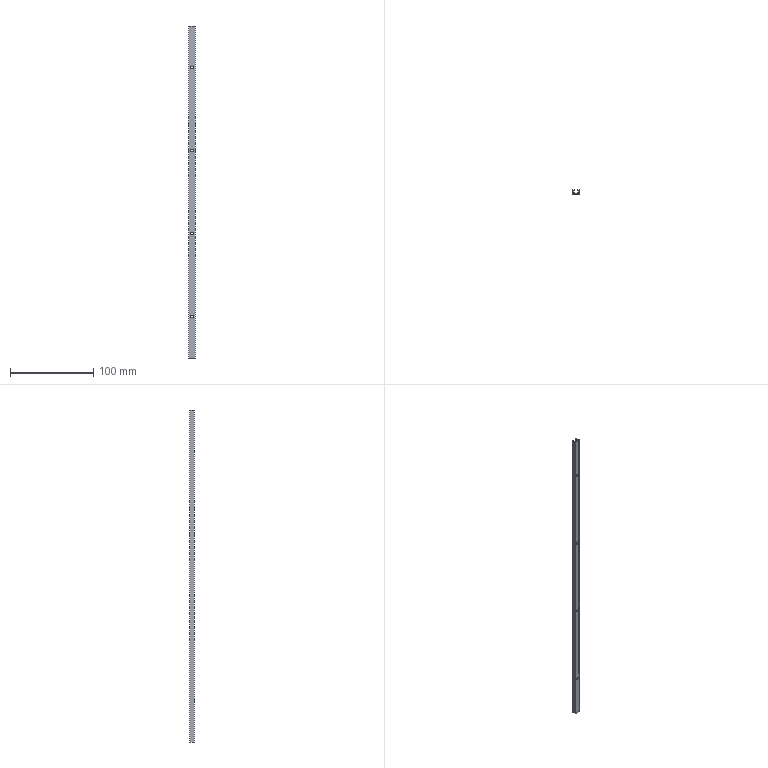Part | SolidWorks | features BaseBody 1 | 1 solid | 26 faces | box 8 x 5 x 400 mm | volume 7551 mm3 | plane 18 | cylinder 8 | commonest cylinder face diameters 3 x8
STEP:
#1=CARTESIAN_POINT('',(0.,0.9,326.5));
#2=VERTEX_POINT('',#1);
#3=CARTESIAN_POINT('',(0.,0.9,323.5));
#4=VERTEX_POINT('',#3);
#5=CARTESIAN_POINT('',(0.,0.9,325.));
#6=DIRECTION('',(0.,-1.,0.));
#7=DIRECTION('',(0.,0.,-1.));
#8=AXIS2_PLACEMENT_3D('',#5,#6,#7);
#9=CIRCLE('',#8,1.5);
#10=EDGE_CURVE('',#2,#4,#9,.T.);
#11=ORIENTED_EDGE('',*,*,#10,.F.);
#12=CARTESIAN_POINT('',(0.,0.,326.5));
#13=VERTEX_POINT('',#12);
#14=CARTESIAN_POINT('',(0.,4.,326.5));
#15=DIRECTION('',(0.,-1.,0.));
#16=VECTOR('',#15,1000.);
#17=LINE('',#14,#16);
#18=EDGE_CURVE('',#2,#13,#17,.T.);
#19=ORIENTED_EDGE('',*,*,#18,.T.);
#20=CARTESIAN_POINT('',(0.,0.,323.5));
#21=VERTEX_POINT('',#20);
#22=CARTESIAN_POINT('',(0.,0.,325.));
#23=DIRECTION('',(0.,1.,0.));
#24=DIRECTION('',(0.,0.,-1.));
#25=AXIS2_PLACEMENT_3D('',#22,#23,#24);
#26=CIRCLE('',#25,1.5);
#27=EDGE_CURVE('',#21,#13,#26,.T.);
#28=ORIENTED_EDGE('',*,*,#27,.F.);
#29=CARTESIAN_POINT('',(0.,4.,323.5));
#30=DIRECTION('',(0.,-1.,0.));
#31=VECTOR('',#30,1000.);
#32=LINE('',#29,#31);
#33=EDGE_CURVE('',#4,#21,#32,.T.);
#34=ORIENTED_EDGE('',*,*,#33,.F.);
#35=EDGE_LOOP('',(#11,#19,#28,#34));
#36=FACE_OUTER_BOUND('',#35,.T.);
#37=CARTESIAN_POINT('',(0.,4.,325.));
#38=DIRECTION('',(0.,-1.,0.));
#39=DIRECTION('',(0.,0.,-1.));
#40=AXIS2_PLACEMENT_3D('',#37,#38,#39);
#41=CYLINDRICAL_SURFACE('',#40,1.5);
#42=ADVANCED_FACE('',(#36),#41,.F.);
#43=CARTESIAN_POINT('',(0.,0.9,226.5));
#44=VERTEX_POINT('',#43);
#45=CARTESIAN_POINT('',(0.,0.9,223.5));
#46=VERTEX_POINT('',#45);
#47=CARTESIAN_POINT('',(0.,0.9,225.));
#48=DIRECTION('',(0.,-1.,0.));
#49=DIRECTION('',(0.,0.,-1.));
#50=AXIS2_PLACEMENT_3D('',#47,#48,#49);
#51=CIRCLE('',#50,1.5);
#52=EDGE_CURVE('',#44,#46,#51,.T.);
#53=ORIENTED_EDGE('',*,*,#52,.F.);
#54=CARTESIAN_POINT('',(0.,0.,226.5));
#55=VERTEX_POINT('',#54);
#56=CARTESIAN_POINT('',(0.,4.,226.5));
#57=DIRECTION('',(0.,-1.,0.));
#58=VECTOR('',#57,1000.);
#59=LINE('',#56,#58);
#60=EDGE_CURVE('',#44,#55,#59,.T.);
#61=ORIENTED_EDGE('',*,*,#60,.T.);
#62=CARTESIAN_POINT('',(0.,0.,223.5));
#63=VERTEX_POINT('',#62);
#64=CARTESIAN_POINT('',(0.,0.,225.));
#65=DIRECTION('',(0.,1.,0.));
#66=DIRECTION('',(0.,0.,-1.));
#67=AXIS2_PLACEMENT_3D('',#64,#65,#66);
#68=CIRCLE('',#67,1.5);
#69=EDGE_CURVE('',#63,#55,#68,.T.);
#70=ORIENTED_EDGE('',*,*,#69,.F.);
#71=CARTESIAN_POINT('',(0.,4.,223.5));
#72=DIRECTION('',(0.,-1.,0.));
#73=VECTOR('',#72,1000.);
#74=LINE('',#71,#73);
#75=EDGE_CURVE('',#46,#63,#74,.T.);
#76=ORIENTED_EDGE('',*,*,#75,.F.);
#77=EDGE_LOOP('',(#53,#61,#70,#76));
#78=FACE_OUTER_BOUND('',#77,.T.);
#79=CARTESIAN_POINT('',(0.,4.,225.));
#80=DIRECTION('',(0.,-1.,0.));
#81=DIRECTION('',(0.,0.,-1.));
#82=AXIS2_PLACEMENT_3D('',#79,#80,#81);
#83=CYLINDRICAL_SURFACE('',#82,1.5);
#84=ADVANCED_FACE('',(#78),#83,.F.);
#85=CARTESIAN_POINT('',(0.,0.9,126.5));
#86=VERTEX_POINT('',#85);
#87=CARTESIAN_POINT('',(0.,0.9,123.5));
#88=VERTEX_POINT('',#87);
#89=CARTESIAN_POINT('',(0.,0.9,125.));
#90=DIRECTION('',(0.,-1.,0.));
#91=DIRECTION('',(0.,0.,-1.));
#92=AXIS2_PLACEMENT_3D('',#89,#90,#91);
#93=CIRCLE('',#92,1.5);
#94=EDGE_CURVE('',#86,#88,#93,.T.);
#95=ORIENTED_EDGE('',*,*,#94,.F.);
#96=CARTESIAN_POINT('',(0.,0.,126.5));
#97=VERTEX_POINT('',#96);
#98=CARTESIAN_POINT('',(0.,4.,126.5));
#99=DIRECTION('',(0.,-1.,0.));
#100=VECTOR('',#99,1000.);
#101=LINE('',#98,#100);
#102=EDGE_CURVE('',#86,#97,#101,.T.);
#103=ORIENTED_EDGE('',*,*,#102,.T.);
#104=CARTESIAN_POINT('',(0.,0.,123.5));
#105=VERTEX_POINT('',#104);
#106=CARTESIAN_POINT('',(0.,0.,125.));
#107=DIRECTION('',(0.,1.,0.));
#108=DIRECTION('',(0.,0.,-1.));
#109=AXIS2_PLACEMENT_3D('',#106,#107,#108);
#110=CIRCLE('',#109,1.5);
#111=EDGE_CURVE('',#105,#97,#110,.T.);
#112=ORIENTED_EDGE('',*,*,#111,.F.);
#113=CARTESIAN_POINT('',(0.,4.,123.5));
#114=DIRECTION('',(0.,-1.,0.));
#115=VECTOR('',#114,1000.);
#116=LINE('',#113,#115);
#117=EDGE_CURVE('',#88,#105,#116,.T.);
#118=ORIENTED_EDGE('',*,*,#117,.F.);
#119=EDGE_LOOP('',(#95,#103,#112,#118));
#120=FACE_OUTER_BOUND('',#119,.T.);
#121=CARTESIAN_POINT('',(0.,4.,125.));
#122=DIRECTION('',(0.,-1.,0.));
#123=DIRECTION('',(0.,0.,-1.));
#124=AXIS2_PLACEMENT_3D('',#121,#122,#123);
#125=CYLINDRICAL_SURFACE('',#124,1.5);
#126=ADVANCED_FACE('',(#120),#125,.F.);
#127=CARTESIAN_POINT('',(0.,0.9,26.5));
#128=VERTEX_POINT('',#127);
#129=CARTESIAN_POINT('',(0.,0.9,23.5));
#130=VERTEX_POINT('',#129);
#131=CARTESIAN_POINT('',(0.,0.9,25.));
#132=DIRECTION('',(0.,-1.,0.));
#133=DIRECTION('',(0.,0.,-1.));
#134=AXIS2_PLACEMENT_3D('',#131,#132,#133);
#135=CIRCLE('',#134,1.5);
#136=EDGE_CURVE('',#128,#130,#135,.T.);
#137=ORIENTED_EDGE('',*,*,#136,.F.);
#138=CARTESIAN_POINT('',(0.,0.,26.5));
#139=VERTEX_POINT('',#138);
#140=CARTESIAN_POINT('',(0.,4.,26.5));
#141=DIRECTION('',(0.,-1.,0.));
#142=VECTOR('',#141,1000.);
#143=LINE('',#140,#142);
#144=EDGE_CURVE('',#128,#139,#143,.T.);
#145=ORIENTED_EDGE('',*,*,#144,.T.);
#146=CARTESIAN_POINT('',(0.,0.,23.5));
#147=VERTEX_POINT('',#146);
#148=CARTESIAN_POINT('',(0.,0.,25.));
#149=DIRECTION('',(0.,1.,0.));
#150=DIRECTION('',(0.,0.,-1.));
#151=AXIS2_PLACEMENT_3D('',#148,#149,#150);
#152=CIRCLE('',#151,1.5);
#153=EDGE_CURVE('',#147,#139,#152,.T.);
#154=ORIENTED_EDGE('',*,*,#153,.F.);
#155=CARTESIAN_POINT('',(0.,4.,23.5));
#156=DIRECTION('',(0.,-1.,0.));
#157=VECTOR('',#156,1000.);
#158=LINE('',#155,#157);
#159=EDGE_CURVE('',#130,#147,#158,.T.);
#160=ORIENTED_EDGE('',*,*,#159,.F.);
#161=EDGE_LOOP('',(#137,#145,#154,#160));
#162=FACE_OUTER_BOUND('',#161,.T.);
#163=CARTESIAN_POINT('',(0.,4.,25.));
#164=DIRECTION('',(0.,-1.,0.));
#165=DIRECTION('',(0.,0.,-1.));
#166=AXIS2_PLACEMENT_3D('',#163,#164,#165);
#167=CYLINDRICAL_SURFACE('',#166,1.5);
#168=ADVANCED_FACE('',(#162),#167,.F.);
#169=ORIENTED_EDGE('',*,*,#27,.T.);
#170=CARTESIAN_POINT('',(0.,0.,325.));
#171=DIRECTION('',(0.,1.,0.));
#172=DIRECTION('',(0.,0.,-1.));
#173=AXIS2_PLACEMENT_3D('',#170,#171,#172);
#174=CIRCLE('',#173,1.5);
#175=EDGE_CURVE('',#13,#21,#174,.T.);
#176=ORIENTED_EDGE('',*,*,#175,.T.);
#177=EDGE_LOOP('',(#169,#176));
#178=FACE_BOUND('',#177,.T.);
#179=ORIENTED_EDGE('',*,*,#69,.T.);
#180=CARTESIAN_POINT('',(0.,0.,225.));
#181=DIRECTION('',(0.,1.,0.));
#182=DIRECTION('',(0.,0.,-1.));
#183=AXIS2_PLACEMENT_3D('',#180,#181,#182);
#184=CIRCLE('',#183,1.5);
#185=EDGE_CURVE('',#55,#63,#184,.T.);
#186=ORIENTED_EDGE('',*,*,#185,.T.);
#187=EDGE_LOOP('',(#179,#186));
#188=FACE_BOUND('',#187,.T.);
#189=ORIENTED_EDGE('',*,*,#111,.T.);
#190=CARTESIAN_POINT('',(0.,0.,125.));
#191=DIRECTION('',(0.,1.,0.));
#192=DIRECTION('',(0.,0.,-1.));
#193=AXIS2_PLACEMENT_3D('',#190,#191,#192);
#194=CIRCLE('',#193,1.5);
#195=EDGE_CURVE('',#97,#105,#194,.T.);
#196=ORIENTED_EDGE('',*,*,#195,.T.);
#197=EDGE_LOOP('',(#189,#196));
#198=FACE_BOUND('',#197,.T.);
#199=ORIENTED_EDGE('',*,*,#153,.T.);
#200=CARTESIAN_POINT('',(0.,0.,25.));
#201=DIRECTION('',(0.,1.,0.));
#202=DIRECTION('',(0.,0.,-1.));
#203=AXIS2_PLACEMENT_3D('',#200,#201,#202);
#204=CIRCLE('',#203,1.5);
#205=EDGE_CURVE('',#139,#147,#204,.T.);
#206=ORIENTED_EDGE('',*,*,#205,.T.);
#207=EDGE_LOOP('',(#199,#206));
#208=FACE_BOUND('',#207,.T.);
#209=CARTESIAN_POINT('',(-4.,0.,-25.));
#210=VERTEX_POINT('',#209);
#211=CARTESIAN_POINT('',(4.,0.,-25.));
#212=VERTEX_POINT('',#211);
#213=CARTESIAN_POINT('',(-4.,0.,-25.));
#214=DIRECTION('',(1.,0.,0.));
#215=VECTOR('',#214,1000.);
#216=LINE('',#213,#215);
#217=EDGE_CURVE('',#210,#212,#216,.T.);
#218=ORIENTED_EDGE('',*,*,#217,.T.);
#219=CARTESIAN_POINT('',(4.,0.,375.));
#220=VERTEX_POINT('',#219);
#221=CARTESIAN_POINT('',(4.,0.,0.));
#222=DIRECTION('',(0.,0.,1.));
#223=VECTOR('',#222,1000.);
#224=LINE('',#221,#223);
#225=EDGE_CURVE('',#212,#220,#224,.T.);
#226=ORIENTED_EDGE('',*,*,#225,.T.);
#227=CARTESIAN_POINT('',(-4.,0.,375.));
#228=VERTEX_POINT('',#227);
#229=CARTESIAN_POINT('',(-4.,0.,375.));
#230=DIRECTION('',(-1.,0.,0.));
#231=VECTOR('',#230,1000.);
#232=LINE('',#229,#231);
#233=EDGE_CURVE('',#220,#228,#232,.T.);
#234=ORIENTED_EDGE('',*,*,#233,.T.);
#235=CARTESIAN_POINT('',(-4.,0.,0.));
#236=DIRECTION('',(0.,0.,-1.));
#237=VECTOR('',#236,1000.);
#238=LINE('',#235,#237);
#239=EDGE_CURVE('',#228,#210,#238,.T.);
#240=ORIENTED_EDGE('',*,*,#239,.T.);
#241=EDGE_LOOP('',(#218,#226,#234,#240));
#242=FACE_OUTER_BOUND('',#241,.T.);
#243=CARTESIAN_POINT('',(-4.,0.,0.));
#244=DIRECTION('',(0.,-1.,0.));
#245=DIRECTION('',(0.,0.,-1.));
#246=AXIS2_PLACEMENT_3D('',#243,#244,#245);
#247=PLANE('',#246);
#248=ADVANCED_FACE('',(#178,#188,#198,#208,#242),#247,.T.);
#249=ORIENTED_EDGE('',*,*,#18,.F.);
#250=CARTESIAN_POINT('',(0.,0.9,325.));
#251=DIRECTION('',(0.,-1.,0.));
#252=DIRECTION('',(0.,0.,-1.));
#253=AXIS2_PLACEMENT_3D('',#250,#251,#252);
#254=CIRCLE('',#253,1.5);
#255=EDGE_CURVE('',#4,#2,#254,.T.);
#256=ORIENTED_EDGE('',*,*,#255,.F.);
#257=ORIENTED_EDGE('',*,*,#33,.T.);
#258=ORIENTED_EDGE('',*,*,#175,.F.);
#259=EDGE_LOOP('',(#249,#256,#257,#258));
#260=FACE_OUTER_BOUND('',#259,.T.);
#261=CARTESIAN_POINT('',(0.,4.,325.));
#262=DIRECTION('',(0.,-1.,0.));
#263=DIRECTION('',(0.,0.,-1.));
#264=AXIS2_PLACEMENT_3D('',#261,#262,#263);
#265=CYLINDRICAL_SURFACE('',#264,1.5);
#266=ADVANCED_FACE('',(#260),#265,.F.);
#267=ORIENTED_EDGE('',*,*,#60,.F.);
#268=CARTESIAN_POINT('',(0.,0.9,225.));
#269=DIRECTION('',(0.,-1.,0.));
#270=DIRECTION('',(0.,0.,-1.));
#271=AXIS2_PLACEMENT_3D('',#268,#269,#270);
#272=CIRCLE('',#271,1.5);
#273=EDGE_CURVE('',#46,#44,#272,.T.);
#274=ORIENTED_EDGE('',*,*,#273,.F.);
#275=ORIENTED_EDGE('',*,*,#75,.T.);
#276=ORIENTED_EDGE('',*,*,#185,.F.);
#277=EDGE_LOOP('',(#267,#274,#275,#276));
#278=FACE_OUTER_BOUND('',#277,.T.);
#279=CARTESIAN_POINT('',(0.,4.,225.));
#280=DIRECTION('',(0.,-1.,0.));
#281=DIRECTION('',(0.,0.,-1.));
#282=AXIS2_PLACEMENT_3D('',#279,#280,#281);
#283=CYLINDRICAL_SURFACE('',#282,1.5);
#284=ADVANCED_FACE('',(#278),#283,.F.);
#285=ORIENTED_EDGE('',*,*,#102,.F.);
#286=CARTESIAN_POINT('',(0.,0.9,125.));
#287=DIRECTION('',(0.,-1.,0.));
#288=DIRECTION('',(0.,0.,-1.));
#289=AXIS2_PLACEMENT_3D('',#286,#287,#288);
#290=CIRCLE('',#289,1.5);
#291=EDGE_CURVE('',#88,#86,#290,.T.);
#292=ORIENTED_EDGE('',*,*,#291,.F.);
#293=ORIENTED_EDGE('',*,*,#117,.T.);
#294=ORIENTED_EDGE('',*,*,#195,.F.);
#295=EDGE_LOOP('',(#285,#292,#293,#294));
#296=FACE_OUTER_BOUND('',#295,.T.);
#297=CARTESIAN_POINT('',(0.,4.,125.));
#298=DIRECTION('',(0.,-1.,0.));
#299=DIRECTION('',(0.,0.,-1.));
#300=AXIS2_PLACEMENT_3D('',#297,#298,#299);
#301=CYLINDRICAL_SURFACE('',#300,1.5);
#302=ADVANCED_FACE('',(#296),#301,.F.);
#303=ORIENTED_EDGE('',*,*,#144,.F.);
#304=CARTESIAN_POINT('',(0.,0.9,25.));
#305=DIRECTION('',(0.,-1.,0.));
#306=DIRECTION('',(0.,0.,-1.));
#307=AXIS2_PLACEMENT_3D('',#304,#305,#306);
#308=CIRCLE('',#307,1.5);
#309=EDGE_CURVE('',#130,#128,#308,.T.);
#310=ORIENTED_EDGE('',*,*,#309,.F.);
#311=ORIENTED_EDGE('',*,*,#159,.T.);
#312=ORIENTED_EDGE('',*,*,#205,.F.);
#313=EDGE_LOOP('',(#303,#310,#311,#312));
#314=FACE_OUTER_BOUND('',#313,.T.);
#315=CARTESIAN_POINT('',(0.,4.,25.));
#316=DIRECTION('',(0.,-1.,0.));
#317=DIRECTION('',(0.,0.,-1.));
#318=AXIS2_PLACEMENT_3D('',#315,#316,#317);
#319=CYLINDRICAL_SURFACE('',#318,1.5);
#320=ADVANCED_FACE('',(#314),#319,.F.);
#321=CARTESIAN_POINT('',(4.,5.,375.));
#322=VERTEX_POINT('',#321);
#323=CARTESIAN_POINT('',(4.,0.,375.));
#324=DIRECTION('',(0.,-1.,0.));
#325=VECTOR('',#324,1000.);
#326=LINE('',#323,#325);
#327=EDGE_CURVE('',#322,#220,#326,.T.);
#328=ORIENTED_EDGE('',*,*,#327,.T.);
#329=ORIENTED_EDGE('',*,*,#225,.F.);
#330=CARTESIAN_POINT('',(4.,5.,-25.));
#331=VERTEX_POINT('',#330);
#332=CARTESIAN_POINT('',(4.,0.,-25.));
#333=DIRECTION('',(0.,1.,0.));
#334=VECTOR('',#333,1000.);
#335=LINE('',#332,#334);
#336=EDGE_CURVE('',#212,#331,#335,.T.);
#337=ORIENTED_EDGE('',*,*,#336,.T.);
#338=CARTESIAN_POINT('',(4.,5.,0.));
#339=DIRECTION('',(0.,0.,1.));
#340=VECTOR('',#339,1000.);
#341=LINE('',#338,#340);
#342=EDGE_CURVE('',#331,#322,#341,.T.);
#343=ORIENTED_EDGE('',*,*,#342,.T.);
#344=EDGE_LOOP('',(#328,#329,#337,#343));
#345=FACE_OUTER_BOUND('',#344,.T.);
#346=CARTESIAN_POINT('',(4.,0.,0.));
#347=DIRECTION('',(1.,0.,0.));
#348=DIRECTION('',(0.,0.,-1.));
#349=AXIS2_PLACEMENT_3D('',#346,#347,#348);
#350=PLANE('',#349);
#351=ADVANCED_FACE('',(#345),#350,.T.);
#352=ORIENTED_EDGE('',*,*,#217,.F.);
#353=CARTESIAN_POINT('',(-4.,5.,-25.));
#354=VERTEX_POINT('',#353);
#355=CARTESIAN_POINT('',(-4.,0.,-25.));
#356=DIRECTION('',(0.,-1.,0.));
#357=VECTOR('',#356,1000.);
#358=LINE('',#355,#357);
#359=EDGE_CURVE('',#354,#210,#358,.T.);
#360=ORIENTED_EDGE('',*,*,#359,.F.);
#361=CARTESIAN_POINT('',(-2.1,5.,-25.));
#362=VERTEX_POINT('',#361);
#363=CARTESIAN_POINT('',(0.,5.,-25.));
#364=DIRECTION('',(-1.,0.,0.));
#365=VECTOR('',#364,1000.);
#366=LINE('',#363,#365);
#367=EDGE_CURVE('',#362,#354,#366,.T.);
#368=ORIENTED_EDGE('',*,*,#367,.F.);
#369=CARTESIAN_POINT('',(-2.1,4.2,-25.));
#370=VERTEX_POINT('',#369);
#371=CARTESIAN_POINT('',(-2.1,4.2,-25.));
#372=DIRECTION('',(0.,1.,0.));
#373=VECTOR('',#372,1000.);
#374=LINE('',#371,#373);
#375=EDGE_CURVE('',#370,#362,#374,.T.);
#376=ORIENTED_EDGE('',*,*,#375,.F.);
#377=CARTESIAN_POINT('',(-2.9,4.2,-25.));
#378=VERTEX_POINT('',#377);
#379=CARTESIAN_POINT('',(-2.9,4.2,-25.));
#380=DIRECTION('',(1.,0.,0.));
#381=VECTOR('',#380,1000.);
#382=LINE('',#379,#381);
#383=EDGE_CURVE('',#378,#370,#382,.T.);
#384=ORIENTED_EDGE('',*,*,#383,.F.);
#385=CARTESIAN_POINT('',(-2.9,1.8,-25.));
#386=VERTEX_POINT('',#385);
#387=CARTESIAN_POINT('',(-2.9,0.,-25.));
#388=DIRECTION('',(0.,1.,0.));
#389=VECTOR('',#388,1000.);
#390=LINE('',#387,#389);
#391=EDGE_CURVE('',#386,#378,#390,.T.);
#392=ORIENTED_EDGE('',*,*,#391,.F.);
#393=CARTESIAN_POINT('',(-2.1,1.8,-25.));
#394=VERTEX_POINT('',#393);
#395=CARTESIAN_POINT('',(-2.1,1.8,-25.));
#396=DIRECTION('',(-1.,0.,0.));
#397=VECTOR('',#396,1000.);
#398=LINE('',#395,#397);
#399=EDGE_CURVE('',#394,#386,#398,.T.);
#400=ORIENTED_EDGE('',*,*,#399,.F.);
#401=CARTESIAN_POINT('',(-2.1,0.9,-25.));
#402=VERTEX_POINT('',#401);
#403=CARTESIAN_POINT('',(-2.1,0.9,-25.));
#404=DIRECTION('',(0.,1.,0.));
#405=VECTOR('',#404,1000.);
#406=LINE('',#403,#405);
#407=EDGE_CURVE('',#402,#394,#406,.T.);
#408=ORIENTED_EDGE('',*,*,#407,.F.);
#409=CARTESIAN_POINT('',(2.1,0.9,-25.));
#410=VERTEX_POINT('',#409);
#411=CARTESIAN_POINT('',(0.,0.9,-25.));
#412=DIRECTION('',(-1.,0.,0.));
#413=VECTOR('',#412,1000.);
#414=LINE('',#411,#413);
#415=EDGE_CURVE('',#410,#402,#414,.T.);
#416=ORIENTED_EDGE('',*,*,#415,.F.);
#417=CARTESIAN_POINT('',(2.1,1.8,-25.));
#418=VERTEX_POINT('',#417);
#419=CARTESIAN_POINT('',(2.1,1.8,-25.));
#420=DIRECTION('',(0.,-1.,0.));
#421=VECTOR('',#420,1000.);
#422=LINE('',#419,#421);
#423=EDGE_CURVE('',#418,#410,#422,.T.);
#424=ORIENTED_EDGE('',*,*,#423,.F.);
#425=CARTESIAN_POINT('',(2.9,1.8,-25.));
#426=VERTEX_POINT('',#425);
#427=CARTESIAN_POINT('',(2.9,1.8,-25.));
#428=DIRECTION('',(-1.,0.,0.));
#429=VECTOR('',#428,1000.);
#430=LINE('',#427,#429);
#431=EDGE_CURVE('',#426,#418,#430,.T.);
#432=ORIENTED_EDGE('',*,*,#431,.F.);
#433=CARTESIAN_POINT('',(2.9,4.2,-25.));
#434=VERTEX_POINT('',#433);
#435=CARTESIAN_POINT('',(2.9,0.,-25.));
#436=DIRECTION('',(0.,-1.,0.));
#437=VECTOR('',#436,1000.);
#438=LINE('',#435,#437);
#439=EDGE_CURVE('',#434,#426,#438,.T.);
#440=ORIENTED_EDGE('',*,*,#439,.F.);
#441=CARTESIAN_POINT('',(2.1,4.2,-25.));
#442=VERTEX_POINT('',#441);
#443=CARTESIAN_POINT('',(2.1,4.2,-25.));
#444=DIRECTION('',(1.,0.,0.));
#445=VECTOR('',#444,1000.);
#446=LINE('',#443,#445);
#447=EDGE_CURVE('',#442,#434,#446,.T.);
#448=ORIENTED_EDGE('',*,*,#447,.F.);
#449=CARTESIAN_POINT('',(2.1,5.,-25.));
#450=VERTEX_POINT('',#449);
#451=CARTESIAN_POINT('',(2.1,5.,-25.));
#452=DIRECTION('',(0.,-1.,0.));
#453=VECTOR('',#452,1000.);
#454=LINE('',#451,#453);
#455=EDGE_CURVE('',#450,#442,#454,.T.);
#456=ORIENTED_EDGE('',*,*,#455,.F.);
#457=CARTESIAN_POINT('',(0.,5.,-25.));
#458=DIRECTION('',(-1.,0.,0.));
#459=VECTOR('',#458,1000.);
#460=LINE('',#457,#459);
#461=EDGE_CURVE('',#331,#450,#460,.T.);
#462=ORIENTED_EDGE('',*,*,#461,.F.);
#463=ORIENTED_EDGE('',*,*,#336,.F.);
#464=EDGE_LOOP('',(#352,#360,#368,#376,#384,#392,#400,#408,#416,#424,#432,#440,#448,#456,#462,#463));
#465=FACE_OUTER_BOUND('',#464,.T.);
#466=CARTESIAN_POINT('',(0.,0.,-25.));
#467=DIRECTION('',(0.,0.,1.));
#468=DIRECTION('',(1.,0.,0.));
#469=AXIS2_PLACEMENT_3D('',#466,#467,#468);
#470=PLANE('',#469);
#471=ADVANCED_FACE('',(#465),#470,.F.);
#472=CARTESIAN_POINT('',(-4.,5.,375.));
#473=VERTEX_POINT('',#472);
#474=CARTESIAN_POINT('',(-4.,5.,375.));
#475=DIRECTION('',(0.,1.,0.));
#476=VECTOR('',#475,1000.);
#477=LINE('',#474,#476);
#478=EDGE_CURVE('',#228,#473,#477,.T.);
#479=ORIENTED_EDGE('',*,*,#478,.T.);
#480=CARTESIAN_POINT('',(-4.,5.,0.));
#481=DIRECTION('',(0.,0.,-1.));
#482=VECTOR('',#481,1000.);
#483=LINE('',#480,#482);
#484=EDGE_CURVE('',#473,#354,#483,.T.);
#485=ORIENTED_EDGE('',*,*,#484,.T.);
#486=ORIENTED_EDGE('',*,*,#359,.T.);
#487=ORIENTED_EDGE('',*,*,#239,.F.);
#488=EDGE_LOOP('',(#479,#485,#486,#487));
#489=FACE_OUTER_BOUND('',#488,.T.);
#490=CARTESIAN_POINT('',(-4.,5.,0.));
#491=DIRECTION('',(-1.,0.,0.));
#492=DIRECTION('',(0.,0.,1.));
#493=AXIS2_PLACEMENT_3D('',#490,#491,#492);
#494=PLANE('',#493);
#495=ADVANCED_FACE('',(#489),#494,.T.);
#496=CARTESIAN_POINT('',(2.1,1.8,375.));
#497=VERTEX_POINT('',#496);
#498=CARTESIAN_POINT('',(2.9,1.8,375.));
#499=VERTEX_POINT('',#498);
#500=CARTESIAN_POINT('',(2.9,1.8,375.));
#501=DIRECTION('',(1.,0.,0.));
#502=VECTOR('',#501,1000.);
#503=LINE('',#500,#502);
#504=EDGE_CURVE('',#497,#499,#503,.T.);
#505=ORIENTED_EDGE('',*,*,#504,.F.);
#506=CARTESIAN_POINT('',(2.1,0.9,375.));
#507=VERTEX_POINT('',#506);
#508=CARTESIAN_POINT('',(2.1,1.8,375.));
#509=DIRECTION('',(0.,1.,0.));
#510=VECTOR('',#509,1000.);
#511=LINE('',#508,#510);
#512=EDGE_CURVE('',#507,#497,#511,.T.);
#513=ORIENTED_EDGE('',*,*,#512,.F.);
#514=CARTESIAN_POINT('',(-2.1,0.9,375.));
#515=VERTEX_POINT('',#514);
#516=CARTESIAN_POINT('',(0.,0.9,375.));
#517=DIRECTION('',(-1.,0.,0.));
#518=VECTOR('',#517,1000.);
#519=LINE('',#516,#518);
#520=EDGE_CURVE('',#507,#515,#519,.T.);
#521=ORIENTED_EDGE('',*,*,#520,.T.);
#522=CARTESIAN_POINT('',(-2.1,1.8,375.));
#523=VERTEX_POINT('',#522);
#524=CARTESIAN_POINT('',(-2.1,0.9,375.));
#525=DIRECTION('',(0.,-1.,0.));
#526=VECTOR('',#525,1000.);
#527=LINE('',#524,#526);
#528=EDGE_CURVE('',#523,#515,#527,.T.);
#529=ORIENTED_EDGE('',*,*,#528,.F.);
#530=CARTESIAN_POINT('',(-2.9,1.8,375.));
#531=VERTEX_POINT('',#530);
#532=CARTESIAN_POINT('',(-2.1,1.8,375.));
#533=DIRECTION('',(1.,0.,0.));
#534=VECTOR('',#533,1000.);
#535=LINE('',#532,#534);
#536=EDGE_CURVE('',#531,#523,#535,.T.);
#537=ORIENTED_EDGE('',*,*,#536,.F.);
#538=CARTESIAN_POINT('',(-2.9,4.2,375.));
#539=VERTEX_POINT('',#538);
#540=CARTESIAN_POINT('',(-2.9,0.,375.));
#541=DIRECTION('',(0.,1.,0.));
#542=VECTOR('',#541,1000.);
#543=LINE('',#540,#542);
#544=EDGE_CURVE('',#531,#539,#543,.T.);
#545=ORIENTED_EDGE('',*,*,#544,.T.);
#546=CARTESIAN_POINT('',(-2.1,4.2,375.));
#547=VERTEX_POINT('',#546);
#548=CARTESIAN_POINT('',(-2.9,4.2,375.));
#549=DIRECTION('',(-1.,0.,0.));
#550=VECTOR('',#549,1000.);
#551=LINE('',#548,#550);
#552=EDGE_CURVE('',#547,#539,#551,.T.);
#553=ORIENTED_EDGE('',*,*,#552,.F.);
#554=CARTESIAN_POINT('',(-2.1,5.,375.));
#555=VERTEX_POINT('',#554);
#556=CARTESIAN_POINT('',(-2.1,4.2,375.));
#557=DIRECTION('',(0.,-1.,0.));
#558=VECTOR('',#557,1000.);
#559=LINE('',#556,#558);
#560=EDGE_CURVE('',#555,#547,#559,.T.);
#561=ORIENTED_EDGE('',*,*,#560,.F.);
#562=CARTESIAN_POINT('',(0.,5.,375.));
#563=DIRECTION('',(-1.,0.,0.));
#564=VECTOR('',#563,1000.);
#565=LINE('',#562,#564);
#566=EDGE_CURVE('',#555,#473,#565,.T.);
#567=ORIENTED_EDGE('',*,*,#566,.T.);
#568=ORIENTED_EDGE('',*,*,#478,.F.);
#569=ORIENTED_EDGE('',*,*,#233,.F.);
#570=ORIENTED_EDGE('',*,*,#327,.F.);
#571=CARTESIAN_POINT('',(2.1,5.,375.));
#572=VERTEX_POINT('',#571);
#573=CARTESIAN_POINT('',(0.,5.,375.));
#574=DIRECTION('',(-1.,0.,0.));
#575=VECTOR('',#574,1000.);
#576=LINE('',#573,#575);
#577=EDGE_CURVE('',#322,#572,#576,.T.);
#578=ORIENTED_EDGE('',*,*,#577,.T.);
#579=CARTESIAN_POINT('',(2.1,4.2,375.));
#580=VERTEX_POINT('',#579);
#581=CARTESIAN_POINT('',(2.1,5.,375.));
#582=DIRECTION('',(0.,1.,0.));
#583=VECTOR('',#582,1000.);
#584=LINE('',#581,#583);
#585=EDGE_CURVE('',#580,#572,#584,.T.);
#586=ORIENTED_EDGE('',*,*,#585,.F.);
#587=CARTESIAN_POINT('',(2.9,4.2,375.));
#588=VERTEX_POINT('',#587);
#589=CARTESIAN_POINT('',(2.1,4.2,375.));
#590=DIRECTION('',(-1.,0.,0.));
#591=VECTOR('',#590,1000.);
#592=LINE('',#589,#591);
#593=EDGE_CURVE('',#588,#580,#592,.T.);
#594=ORIENTED_EDGE('',*,*,#593,.F.);
#595=CARTESIAN_POINT('',(2.9,0.,375.));
#596=DIRECTION('',(0.,-1.,0.));
#597=VECTOR('',#596,1000.);
#598=LINE('',#595,#597);
#599=EDGE_CURVE('',#588,#499,#598,.T.);
#600=ORIENTED_EDGE('',*,*,#599,.T.);
#601=EDGE_LOOP('',(#505,#513,#521,#529,#537,#545,#553,#561,#567,#568,#569,#570,#578,#586,#594,#600));
#602=FACE_OUTER_BOUND('',#601,.T.);
#603=CARTESIAN_POINT('',(0.,0.,375.));
#604=DIRECTION('',(0.,0.,1.));
#605=DIRECTION('',(1.,0.,0.));
#606=AXIS2_PLACEMENT_3D('',#603,#604,#605);
#607=PLANE('',#606);
#608=ADVANCED_FACE('',(#602),#607,.T.);
#609=ORIENTED_EDGE('',*,*,#255,.T.);
#610=ORIENTED_EDGE('',*,*,#10,.T.);
#611=EDGE_LOOP('',(#609,#610));
#612=FACE_BOUND('',#611,.T.);
#613=ORIENTED_EDGE('',*,*,#273,.T.);
#614=ORIENTED_EDGE('',*,*,#52,.T.);
#615=EDGE_LOOP('',(#613,#614));
#616=FACE_BOUND('',#615,.T.);
#617=ORIENTED_EDGE('',*,*,#291,.T.);
#618=ORIENTED_EDGE('',*,*,#94,.T.);
#619=EDGE_LOOP('',(#617,#618));
#620=FACE_BOUND('',#619,.T.);
#621=ORIENTED_EDGE('',*,*,#309,.T.);
#622=ORIENTED_EDGE('',*,*,#136,.T.);
#623=EDGE_LOOP('',(#621,#622));
#624=FACE_BOUND('',#623,.T.);
#625=ORIENTED_EDGE('',*,*,#415,.T.);
#626=CARTESIAN_POINT('',(-2.1,0.9,0.));
#627=DIRECTION('',(0.,0.,1.));
#628=VECTOR('',#627,1000.);
#629=LINE('',#626,#628);
#630=EDGE_CURVE('',#402,#515,#629,.T.);
#631=ORIENTED_EDGE('',*,*,#630,.T.);
#632=ORIENTED_EDGE('',*,*,#520,.F.);
#633=CARTESIAN_POINT('',(2.1,0.9,0.));
#634=DIRECTION('',(0.,0.,-1.));
#635=VECTOR('',#634,1000.);
#636=LINE('',#633,#635);
#637=EDGE_CURVE('',#507,#410,#636,.T.);
#638=ORIENTED_EDGE('',*,*,#637,.T.);
#639=EDGE_LOOP('',(#625,#631,#632,#638));
#640=FACE_OUTER_BOUND('',#639,.T.);
#641=CARTESIAN_POINT('',(2.1,0.9,0.));
#642=DIRECTION('',(0.,1.,0.));
#643=DIRECTION('',(0.,0.,1.));
#644=AXIS2_PLACEMENT_3D('',#641,#642,#643);
#645=PLANE('',#644);
#646=ADVANCED_FACE('',(#612,#616,#620,#624,#640),#645,.T.);
#647=ORIENTED_EDGE('',*,*,#577,.F.);
#648=ORIENTED_EDGE('',*,*,#342,.F.);
#649=ORIENTED_EDGE('',*,*,#461,.T.);
#650=CARTESIAN_POINT('',(2.1,5.,0.));
#651=DIRECTION('',(0.,0.,1.));
#652=VECTOR('',#651,1000.);
#653=LINE('',#650,#652);
#654=EDGE_CURVE('',#450,#572,#653,.T.);
#655=ORIENTED_EDGE('',*,*,#654,.T.);
#656=EDGE_LOOP('',(#647,#648,#649,#655));
#657=FACE_OUTER_BOUND('',#656,.T.);
#658=CARTESIAN_POINT('',(4.,5.,0.));
#659=DIRECTION('',(0.,1.,0.));
#660=DIRECTION('',(0.,0.,1.));
#661=AXIS2_PLACEMENT_3D('',#658,#659,#660);
#662=PLANE('',#661);
#663=ADVANCED_FACE('',(#657),#662,.T.);
#664=ORIENTED_EDGE('',*,*,#566,.F.);
#665=CARTESIAN_POINT('',(-2.1,5.,0.));
#666=DIRECTION('',(0.,0.,-1.));
#667=VECTOR('',#666,1000.);
#668=LINE('',#665,#667);
#669=EDGE_CURVE('',#555,#362,#668,.T.);
#670=ORIENTED_EDGE('',*,*,#669,.T.);
#671=ORIENTED_EDGE('',*,*,#367,.T.);
#672=ORIENTED_EDGE('',*,*,#484,.F.);
#673=EDGE_LOOP('',(#664,#670,#671,#672));
#674=FACE_OUTER_BOUND('',#673,.T.);
#675=CARTESIAN_POINT('',(-2.1,5.,0.));
#676=DIRECTION('',(0.,1.,0.));
#677=DIRECTION('',(0.,0.,1.));
#678=AXIS2_PLACEMENT_3D('',#675,#676,#677);
#679=PLANE('',#678);
#680=ADVANCED_FACE('',(#674),#679,.T.);
#681=ORIENTED_EDGE('',*,*,#544,.F.);
#682=CARTESIAN_POINT('',(-2.9,1.8,0.));
#683=DIRECTION('',(0.,0.,-1.));
#684=VECTOR('',#683,1000.);
#685=LINE('',#682,#684);
#686=EDGE_CURVE('',#531,#386,#685,.T.);
#687=ORIENTED_EDGE('',*,*,#686,.T.);
#688=ORIENTED_EDGE('',*,*,#391,.T.);
#689=CARTESIAN_POINT('',(-2.9,4.2,0.));
#690=DIRECTION('',(0.,0.,1.));
#691=VECTOR('',#690,1000.);
#692=LINE('',#689,#691);
#693=EDGE_CURVE('',#378,#539,#692,.T.);
#694=ORIENTED_EDGE('',*,*,#693,.T.);
#695=EDGE_LOOP('',(#681,#687,#688,#694));
#696=FACE_OUTER_BOUND('',#695,.T.);
#697=CARTESIAN_POINT('',(-2.9,1.8,0.));
#698=DIRECTION('',(1.,0.,0.));
#699=DIRECTION('',(0.,0.,-1.));
#700=AXIS2_PLACEMENT_3D('',#697,#698,#699);
#701=PLANE('',#700);
#702=ADVANCED_FACE('',(#696),#701,.T.);
#703=ORIENTED_EDGE('',*,*,#599,.F.);
#704=CARTESIAN_POINT('',(2.9,4.2,0.));
#705=DIRECTION('',(0.,0.,-1.));
#706=VECTOR('',#705,1000.);
#707=LINE('',#704,#706);
#708=EDGE_CURVE('',#588,#434,#707,.T.);
#709=ORIENTED_EDGE('',*,*,#708,.T.);
#710=ORIENTED_EDGE('',*,*,#439,.T.);
#711=CARTESIAN_POINT('',(2.9,1.8,0.));
#712=DIRECTION('',(0.,0.,1.));
#713=VECTOR('',#712,1000.);
#714=LINE('',#711,#713);
#715=EDGE_CURVE('',#426,#499,#714,.T.);
#716=ORIENTED_EDGE('',*,*,#715,.T.);
#717=EDGE_LOOP('',(#703,#709,#710,#716));
#718=FACE_OUTER_BOUND('',#717,.T.);
#719=CARTESIAN_POINT('',(2.9,4.2,0.));
#720=DIRECTION('',(-1.,0.,0.));
#721=DIRECTION('',(0.,0.,1.));
#722=AXIS2_PLACEMENT_3D('',#719,#720,#721);
#723=PLANE('',#722);
#724=ADVANCED_FACE('',(#718),#723,.T.);
#725=ORIENTED_EDGE('',*,*,#528,.T.);
#726=ORIENTED_EDGE('',*,*,#630,.F.);
#727=ORIENTED_EDGE('',*,*,#407,.T.);
#728=CARTESIAN_POINT('',(-2.1,1.8,0.));
#729=DIRECTION('',(0.,0.,1.));
#730=VECTOR('',#729,1000.);
#731=LINE('',#728,#730);
#732=EDGE_CURVE('',#394,#523,#731,.T.);
#733=ORIENTED_EDGE('',*,*,#732,.T.);
#734=EDGE_LOOP('',(#725,#726,#727,#733));
#735=FACE_OUTER_BOUND('',#734,.T.);
#736=CARTESIAN_POINT('',(-2.1,0.9,0.));
#737=DIRECTION('',(1.,0.,0.));
#738=DIRECTION('',(0.,0.,-1.));
#739=AXIS2_PLACEMENT_3D('',#736,#737,#738);
#740=PLANE('',#739);
#741=ADVANCED_FACE('',(#735),#740,.T.);
#742=ORIENTED_EDGE('',*,*,#512,.T.);
#743=CARTESIAN_POINT('',(2.1,1.8,0.));
#744=DIRECTION('',(0.,0.,-1.));
#745=VECTOR('',#744,1000.);
#746=LINE('',#743,#745);
#747=EDGE_CURVE('',#497,#418,#746,.T.);
#748=ORIENTED_EDGE('',*,*,#747,.T.);
#749=ORIENTED_EDGE('',*,*,#423,.T.);
#750=ORIENTED_EDGE('',*,*,#637,.F.);
#751=EDGE_LOOP('',(#742,#748,#749,#750));
#752=FACE_OUTER_BOUND('',#751,.T.);
#753=CARTESIAN_POINT('',(2.1,1.8,0.));
#754=DIRECTION('',(-1.,0.,0.));
#755=DIRECTION('',(0.,0.,1.));
#756=AXIS2_PLACEMENT_3D('',#753,#754,#755);
#757=PLANE('',#756);
#758=ADVANCED_FACE('',(#752),#757,.T.);
#759=ORIENTED_EDGE('',*,*,#585,.T.);
#760=ORIENTED_EDGE('',*,*,#654,.F.);
#761=ORIENTED_EDGE('',*,*,#455,.T.);
#762=CARTESIAN_POINT('',(2.1,4.2,0.));
#763=DIRECTION('',(0.,0.,1.));
#764=VECTOR('',#763,1000.);
#765=LINE('',#762,#764);
#766=EDGE_CURVE('',#442,#580,#765,.T.);
#767=ORIENTED_EDGE('',*,*,#766,.T.);
#768=EDGE_LOOP('',(#759,#760,#761,#767));
#769=FACE_OUTER_BOUND('',#768,.T.);
#770=CARTESIAN_POINT('',(2.1,5.,0.));
#771=DIRECTION('',(-1.,0.,0.));
#772=DIRECTION('',(0.,0.,1.));
#773=AXIS2_PLACEMENT_3D('',#770,#771,#772);
#774=PLANE('',#773);
#775=ADVANCED_FACE('',(#769),#774,.T.);
#776=ORIENTED_EDGE('',*,*,#560,.T.);
#777=CARTESIAN_POINT('',(-2.1,4.2,0.));
#778=DIRECTION('',(0.,0.,-1.));
#779=VECTOR('',#778,1000.);
#780=LINE('',#777,#779);
#781=EDGE_CURVE('',#547,#370,#780,.T.);
#782=ORIENTED_EDGE('',*,*,#781,.T.);
#783=ORIENTED_EDGE('',*,*,#375,.T.);
#784=ORIENTED_EDGE('',*,*,#669,.F.);
#785=EDGE_LOOP('',(#776,#782,#783,#784));
#786=FACE_OUTER_BOUND('',#785,.T.);
#787=CARTESIAN_POINT('',(-2.1,4.2,0.));
#788=DIRECTION('',(1.,0.,0.));
#789=DIRECTION('',(0.,0.,-1.));
#790=AXIS2_PLACEMENT_3D('',#787,#788,#789);
#791=PLANE('',#790);
#792=ADVANCED_FACE('',(#786),#791,.T.);
#793=ORIENTED_EDGE('',*,*,#536,.T.);
#794=ORIENTED_EDGE('',*,*,#732,.F.);
#795=ORIENTED_EDGE('',*,*,#399,.T.);
#796=ORIENTED_EDGE('',*,*,#686,.F.);
#797=EDGE_LOOP('',(#793,#794,#795,#796));
#798=FACE_OUTER_BOUND('',#797,.T.);
#799=CARTESIAN_POINT('',(-2.1,1.8,0.));
#800=DIRECTION('',(0.,1.,0.));
#801=DIRECTION('',(0.,0.,1.));
#802=AXIS2_PLACEMENT_3D('',#799,#800,#801);
#803=PLANE('',#802);
#804=ADVANCED_FACE('',(#798),#803,.T.);
#805=ORIENTED_EDGE('',*,*,#552,.T.);
#806=ORIENTED_EDGE('',*,*,#693,.F.);
#807=ORIENTED_EDGE('',*,*,#383,.T.);
#808=ORIENTED_EDGE('',*,*,#781,.F.);
#809=EDGE_LOOP('',(#805,#806,#807,#808));
#810=FACE_OUTER_BOUND('',#809,.T.);
#811=CARTESIAN_POINT('',(-2.9,4.2,0.));
#812=DIRECTION('',(0.,-1.,0.));
#813=DIRECTION('',(0.,0.,-1.));
#814=AXIS2_PLACEMENT_3D('',#811,#812,#813);
#815=PLANE('',#814);
#816=ADVANCED_FACE('',(#810),#815,.T.);
#817=ORIENTED_EDGE('',*,*,#593,.T.);
#818=ORIENTED_EDGE('',*,*,#766,.F.);
#819=ORIENTED_EDGE('',*,*,#447,.T.);
#820=ORIENTED_EDGE('',*,*,#708,.F.);
#821=EDGE_LOOP('',(#817,#818,#819,#820));
#822=FACE_OUTER_BOUND('',#821,.T.);
#823=CARTESIAN_POINT('',(2.1,4.2,0.));
#824=DIRECTION('',(0.,-1.,0.));
#825=DIRECTION('',(0.,0.,-1.));
#826=AXIS2_PLACEMENT_3D('',#823,#824,#825);
#827=PLANE('',#826);
#828=ADVANCED_FACE('',(#822),#827,.T.);
#829=ORIENTED_EDGE('',*,*,#504,.T.);
#830=ORIENTED_EDGE('',*,*,#715,.F.);
#831=ORIENTED_EDGE('',*,*,#431,.T.);
#832=ORIENTED_EDGE('',*,*,#747,.F.);
#833=EDGE_LOOP('',(#829,#830,#831,#832));
#834=FACE_OUTER_BOUND('',#833,.T.);
#835=CARTESIAN_POINT('',(2.9,1.8,0.));
#836=DIRECTION('',(0.,1.,0.));
#837=DIRECTION('',(0.,0.,1.));
#838=AXIS2_PLACEMENT_3D('',#835,#836,#837);
#839=PLANE('',#838);
#840=ADVANCED_FACE('',(#834),#839,.T.);
#841=CLOSED_SHELL('',(#42,#84,#126,#168,#248,#266,#284,#302,#320,#351,#471,#495,#608,#646,#663,#680,#702,#724,#741,#758,#775,#792,#804,#816,#828,#840));
#842=MANIFOLD_SOLID_BREP('',#841);
#843=CARTESIAN_POINT('',(0.,0.,0.));
#844=DIRECTION('',(0.,0.,1.));
#845=DIRECTION('',(1.,0.,0.));
#846=AXIS2_PLACEMENT_3D('',#843,#844,#845);
#847=(LENGTH_UNIT()NAMED_UNIT(*)SI_UNIT(.MILLI.,.METRE.));
#848=UNCERTAINTY_MEASURE_WITH_UNIT(LENGTH_MEASURE(0.00001),#847,'','');
#849=(NAMED_UNIT(*)PLANE_ANGLE_UNIT()SI_UNIT($,.RADIAN.));
#850=(NAMED_UNIT(*)SI_UNIT($,.STERADIAN.)SOLID_ANGLE_UNIT());
#851=(GEOMETRIC_REPRESENTATION_CONTEXT(3)GLOBAL_UNCERTAINTY_ASSIGNED_CONTEXT((#848))GLOBAL_UNIT_ASSIGNED_CONTEXT((#847,#849,#850))REPRESENTATION_CONTEXT('',''));
#852=ADVANCED_BREP_SHAPE_REPRESENTATION('',(#842,#846),#851);